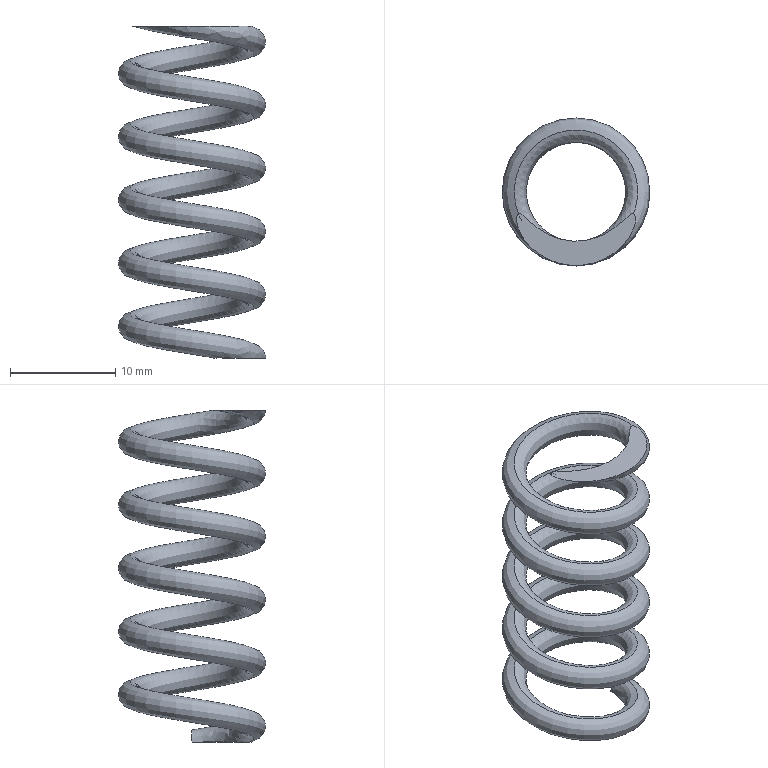Part | SolidWorks | features BaseBody 1 | 1 solid | 5 faces | box 14 x 14 x 31.5 mm | volume 795.453 mm3 | plane 3 | spline 2